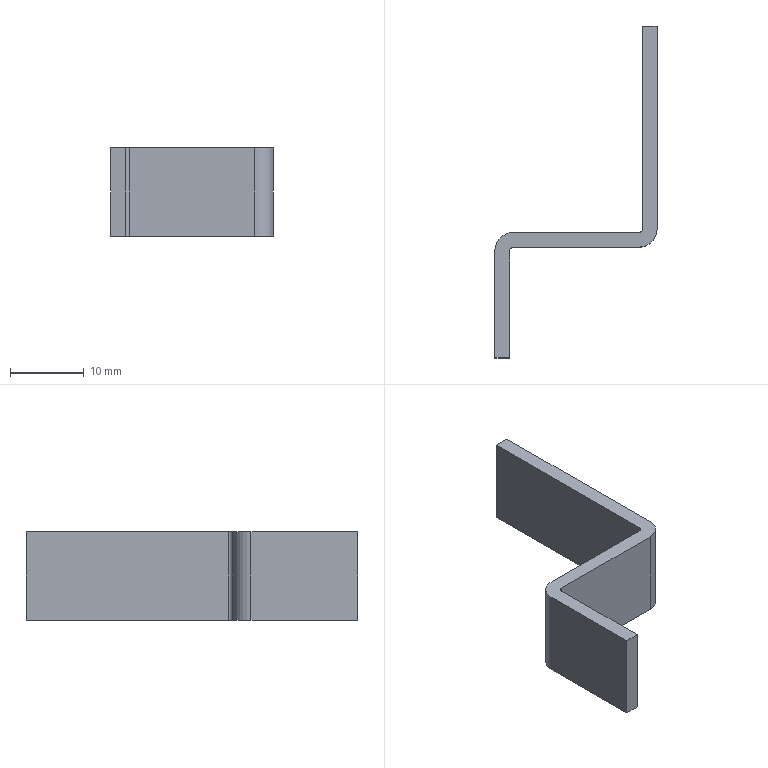Part | STEP file | Clip | 1 solid | 14 faces | box 22 x 45 x 12 mm | volume 1529 mm3 | plane 10 | cylinder 4 | commonest cylinder face diameters 1 x2 5 x2
STEP:
#1=CARTESIAN_POINT('',(0.,-1.053,12.));
#2=VERTEX_POINT('',#1);
#3=CARTESIAN_POINT('',(0.,-28.553,12.));
#4=VERTEX_POINT('',#3);
#5=CARTESIAN_POINT('',(0.,-1.053,12.));
#6=DIRECTION('',(0.,-1.,0.));
#7=VECTOR('',#6,1000.);
#8=LINE('',#5,#7);
#9=EDGE_CURVE('',#2,#4,#8,.T.);
#10=ORIENTED_EDGE('',*,*,#9,.T.);
#11=CARTESIAN_POINT('',(0.,-28.553,0.));
#12=VERTEX_POINT('',#11);
#13=CARTESIAN_POINT('',(0.,-28.553,12.));
#14=DIRECTION('',(0.,0.,-1.));
#15=VECTOR('',#14,1000.);
#16=LINE('',#13,#15);
#17=EDGE_CURVE('',#4,#12,#16,.T.);
#18=ORIENTED_EDGE('',*,*,#17,.T.);
#19=CARTESIAN_POINT('',(0.,-1.053,0.));
#20=VERTEX_POINT('',#19);
#21=CARTESIAN_POINT('',(0.,-1.053,0.));
#22=DIRECTION('',(0.,1.,0.));
#23=VECTOR('',#22,1000.);
#24=LINE('',#21,#23);
#25=EDGE_CURVE('',#12,#20,#24,.T.);
#26=ORIENTED_EDGE('',*,*,#25,.T.);
#27=CARTESIAN_POINT('',(0.,-1.053,12.));
#28=DIRECTION('',(0.,0.,1.));
#29=VECTOR('',#28,1000.);
#30=LINE('',#27,#29);
#31=EDGE_CURVE('',#20,#2,#30,.T.);
#32=ORIENTED_EDGE('',*,*,#31,.T.);
#33=EDGE_LOOP('',(#10,#18,#26,#32));
#34=FACE_OUTER_BOUND('',#33,.T.);
#35=CARTESIAN_POINT('',(0.,-1.053,12.));
#36=DIRECTION('',(1.,0.,0.));
#37=DIRECTION('',(0.,1.,0.));
#38=AXIS2_PLACEMENT_3D('',#35,#36,#37);
#39=PLANE('',#38);
#40=ADVANCED_FACE('',(#34),#39,.T.);
#41=CARTESIAN_POINT('',(-2.5,-31.053,12.));
#42=VERTEX_POINT('',#41);
#43=CARTESIAN_POINT('',(-2.5,-28.553,12.));
#44=DIRECTION('',(0.,0.,-1.));
#45=DIRECTION('',(-1.,0.,0.));
#46=AXIS2_PLACEMENT_3D('',#43,#44,#45);
#47=CIRCLE('',#46,2.5);
#48=EDGE_CURVE('',#4,#42,#47,.T.);
#49=ORIENTED_EDGE('',*,*,#48,.T.);
#50=CARTESIAN_POINT('',(-2.5,-31.053,0.));
#51=VERTEX_POINT('',#50);
#52=CARTESIAN_POINT('',(-2.5,-31.053,12.));
#53=DIRECTION('',(0.,0.,-1.));
#54=VECTOR('',#53,1000.);
#55=LINE('',#52,#54);
#56=EDGE_CURVE('',#42,#51,#55,.T.);
#57=ORIENTED_EDGE('',*,*,#56,.T.);
#58=CARTESIAN_POINT('',(-2.5,-28.553,0.));
#59=DIRECTION('',(0.,0.,1.));
#60=DIRECTION('',(-1.,0.,0.));
#61=AXIS2_PLACEMENT_3D('',#58,#59,#60);
#62=CIRCLE('',#61,2.5);
#63=EDGE_CURVE('',#51,#12,#62,.T.);
#64=ORIENTED_EDGE('',*,*,#63,.T.);
#65=ORIENTED_EDGE('',*,*,#17,.F.);
#66=EDGE_LOOP('',(#49,#57,#64,#65));
#67=FACE_OUTER_BOUND('',#66,.T.);
#68=CARTESIAN_POINT('',(-2.5,-28.553,12.));
#69=DIRECTION('',(0.,0.,-1.));
#70=DIRECTION('',(-1.,0.,0.));
#71=AXIS2_PLACEMENT_3D('',#68,#69,#70);
#72=CYLINDRICAL_SURFACE('',#71,2.5);
#73=ADVANCED_FACE('',(#67),#72,.T.);
#74=CARTESIAN_POINT('',(-2.,-28.553,12.));
#75=VERTEX_POINT('',#74);
#76=CARTESIAN_POINT('',(-2.,-1.053,12.));
#77=VERTEX_POINT('',#76);
#78=CARTESIAN_POINT('',(-2.,-31.553,12.));
#79=DIRECTION('',(0.,1.,0.));
#80=VECTOR('',#79,1000.);
#81=LINE('',#78,#80);
#82=EDGE_CURVE('',#75,#77,#81,.T.);
#83=ORIENTED_EDGE('',*,*,#82,.F.);
#84=CARTESIAN_POINT('',(-2.5,-29.053,12.));
#85=VERTEX_POINT('',#84);
#86=CARTESIAN_POINT('',(-2.5,-28.553,12.));
#87=DIRECTION('',(0.,0.,-1.));
#88=DIRECTION('',(-1.,0.,0.));
#89=AXIS2_PLACEMENT_3D('',#86,#87,#88);
#90=CIRCLE('',#89,0.5);
#91=EDGE_CURVE('',#75,#85,#90,.T.);
#92=ORIENTED_EDGE('',*,*,#91,.T.);
#93=CARTESIAN_POINT('',(-19.5,-29.053,12.));
#94=VERTEX_POINT('',#93);
#95=CARTESIAN_POINT('',(-2.,-29.053,12.));
#96=DIRECTION('',(-1.,0.,0.));
#97=VECTOR('',#96,1000.);
#98=LINE('',#95,#97);
#99=EDGE_CURVE('',#85,#94,#98,.T.);
#100=ORIENTED_EDGE('',*,*,#99,.T.);
#101=CARTESIAN_POINT('',(-22.,-31.553,12.));
#102=VERTEX_POINT('',#101);
#103=CARTESIAN_POINT('',(-19.5,-31.553,12.));
#104=DIRECTION('',(0.,0.,1.));
#105=DIRECTION('',(-1.,0.,0.));
#106=AXIS2_PLACEMENT_3D('',#103,#104,#105);
#107=CIRCLE('',#106,2.5);
#108=EDGE_CURVE('',#94,#102,#107,.T.);
#109=ORIENTED_EDGE('',*,*,#108,.T.);
#110=CARTESIAN_POINT('',(-22.,-46.053,12.));
#111=VERTEX_POINT('',#110);
#112=CARTESIAN_POINT('',(-22.,-29.053,12.));
#113=DIRECTION('',(0.,-1.,0.));
#114=VECTOR('',#113,1000.);
#115=LINE('',#112,#114);
#116=EDGE_CURVE('',#102,#111,#115,.T.);
#117=ORIENTED_EDGE('',*,*,#116,.T.);
#118=CARTESIAN_POINT('',(-20.,-46.053,12.));
#119=VERTEX_POINT('',#118);
#120=CARTESIAN_POINT('',(-20.,-46.053,12.));
#121=DIRECTION('',(-1.,0.,0.));
#122=VECTOR('',#121,1000.);
#123=LINE('',#120,#122);
#124=EDGE_CURVE('',#119,#111,#123,.T.);
#125=ORIENTED_EDGE('',*,*,#124,.F.);
#126=CARTESIAN_POINT('',(-20.,-31.553,12.));
#127=VERTEX_POINT('',#126);
#128=CARTESIAN_POINT('',(-20.,-31.053,12.));
#129=DIRECTION('',(0.,-1.,0.));
#130=VECTOR('',#129,1000.);
#131=LINE('',#128,#130);
#132=EDGE_CURVE('',#127,#119,#131,.T.);
#133=ORIENTED_EDGE('',*,*,#132,.F.);
#134=CARTESIAN_POINT('',(-19.5,-31.053,12.));
#135=VERTEX_POINT('',#134);
#136=CARTESIAN_POINT('',(-19.5,-31.553,12.));
#137=DIRECTION('',(0.,0.,-1.));
#138=DIRECTION('',(-1.,0.,0.));
#139=AXIS2_PLACEMENT_3D('',#136,#137,#138);
#140=CIRCLE('',#139,0.5);
#141=EDGE_CURVE('',#127,#135,#140,.T.);
#142=ORIENTED_EDGE('',*,*,#141,.T.);
#143=CARTESIAN_POINT('',(-20.,-31.053,12.));
#144=DIRECTION('',(-1.,0.,0.));
#145=VECTOR('',#144,1000.);
#146=LINE('',#143,#145);
#147=EDGE_CURVE('',#42,#135,#146,.T.);
#148=ORIENTED_EDGE('',*,*,#147,.F.);
#149=ORIENTED_EDGE('',*,*,#48,.F.);
#150=ORIENTED_EDGE('',*,*,#9,.F.);
#151=CARTESIAN_POINT('',(-19.5,-1.053,12.));
#152=DIRECTION('',(1.,0.,0.));
#153=VECTOR('',#152,1000.);
#154=LINE('',#151,#153);
#155=EDGE_CURVE('',#77,#2,#154,.T.);
#156=ORIENTED_EDGE('',*,*,#155,.F.);
#157=EDGE_LOOP('',(#83,#92,#100,#109,#117,#125,#133,#142,#148,#149,#150,#156));
#158=FACE_OUTER_BOUND('',#157,.T.);
#159=CARTESIAN_POINT('',(-19.5,-31.553,12.));
#160=DIRECTION('',(0.,0.,-1.));
#161=DIRECTION('',(-1.,0.,0.));
#162=AXIS2_PLACEMENT_3D('',#159,#160,#161);
#163=PLANE('',#162);
#164=ADVANCED_FACE('',(#158),#163,.F.);
#165=ORIENTED_EDGE('',*,*,#155,.T.);
#166=ORIENTED_EDGE('',*,*,#31,.F.);
#167=CARTESIAN_POINT('',(-2.,-1.053,0.));
#168=VERTEX_POINT('',#167);
#169=CARTESIAN_POINT('',(-2.,-1.053,0.));
#170=DIRECTION('',(-1.,0.,0.));
#171=VECTOR('',#170,1000.);
#172=LINE('',#169,#171);
#173=EDGE_CURVE('',#20,#168,#172,.T.);
#174=ORIENTED_EDGE('',*,*,#173,.T.);
#175=CARTESIAN_POINT('',(-2.,-1.053,12.));
#176=DIRECTION('',(0.,0.,1.));
#177=VECTOR('',#176,1000.);
#178=LINE('',#175,#177);
#179=EDGE_CURVE('',#168,#77,#178,.T.);
#180=ORIENTED_EDGE('',*,*,#179,.T.);
#181=EDGE_LOOP('',(#165,#166,#174,#180));
#182=FACE_OUTER_BOUND('',#181,.T.);
#183=CARTESIAN_POINT('',(-2.,-1.053,12.));
#184=DIRECTION('',(0.,1.,0.));
#185=DIRECTION('',(-1.,0.,0.));
#186=AXIS2_PLACEMENT_3D('',#183,#184,#185);
#187=PLANE('',#186);
#188=ADVANCED_FACE('',(#182),#187,.T.);
#189=CARTESIAN_POINT('',(-2.,-28.553,0.));
#190=VERTEX_POINT('',#189);
#191=CARTESIAN_POINT('',(-2.,-29.053,0.));
#192=DIRECTION('',(0.,1.,0.));
#193=VECTOR('',#192,1000.);
#194=LINE('',#191,#193);
#195=EDGE_CURVE('',#190,#168,#194,.T.);
#196=ORIENTED_EDGE('',*,*,#195,.T.);
#197=ORIENTED_EDGE('',*,*,#173,.F.);
#198=ORIENTED_EDGE('',*,*,#25,.F.);
#199=ORIENTED_EDGE('',*,*,#63,.F.);
#200=CARTESIAN_POINT('',(-19.5,-31.053,0.));
#201=VERTEX_POINT('',#200);
#202=CARTESIAN_POINT('',(-20.,-31.053,0.));
#203=DIRECTION('',(1.,0.,0.));
#204=VECTOR('',#203,1000.);
#205=LINE('',#202,#204);
#206=EDGE_CURVE('',#201,#51,#205,.T.);
#207=ORIENTED_EDGE('',*,*,#206,.F.);
#208=CARTESIAN_POINT('',(-20.,-31.553,0.));
#209=VERTEX_POINT('',#208);
#210=CARTESIAN_POINT('',(-19.5,-31.553,0.));
#211=DIRECTION('',(0.,0.,1.));
#212=DIRECTION('',(-1.,0.,0.));
#213=AXIS2_PLACEMENT_3D('',#210,#211,#212);
#214=CIRCLE('',#213,0.5);
#215=EDGE_CURVE('',#201,#209,#214,.T.);
#216=ORIENTED_EDGE('',*,*,#215,.T.);
#217=CARTESIAN_POINT('',(-20.,-46.053,0.));
#218=VERTEX_POINT('',#217);
#219=CARTESIAN_POINT('',(-20.,-31.053,0.));
#220=DIRECTION('',(0.,1.,0.));
#221=VECTOR('',#220,1000.);
#222=LINE('',#219,#221);
#223=EDGE_CURVE('',#218,#209,#222,.T.);
#224=ORIENTED_EDGE('',*,*,#223,.F.);
#225=CARTESIAN_POINT('',(-22.,-46.053,0.));
#226=VERTEX_POINT('',#225);
#227=CARTESIAN_POINT('',(-20.,-46.053,0.));
#228=DIRECTION('',(1.,0.,0.));
#229=VECTOR('',#228,1000.);
#230=LINE('',#227,#229);
#231=EDGE_CURVE('',#226,#218,#230,.T.);
#232=ORIENTED_EDGE('',*,*,#231,.F.);
#233=CARTESIAN_POINT('',(-22.,-31.553,0.));
#234=VERTEX_POINT('',#233);
#235=CARTESIAN_POINT('',(-22.,-31.553,0.));
#236=DIRECTION('',(0.,1.,0.));
#237=VECTOR('',#236,1000.);
#238=LINE('',#235,#237);
#239=EDGE_CURVE('',#226,#234,#238,.T.);
#240=ORIENTED_EDGE('',*,*,#239,.T.);
#241=CARTESIAN_POINT('',(-19.5,-29.053,0.));
#242=VERTEX_POINT('',#241);
#243=CARTESIAN_POINT('',(-19.5,-31.553,0.));
#244=DIRECTION('',(0.,0.,-1.));
#245=DIRECTION('',(-1.,0.,0.));
#246=AXIS2_PLACEMENT_3D('',#243,#244,#245);
#247=CIRCLE('',#246,2.5);
#248=EDGE_CURVE('',#234,#242,#247,.T.);
#249=ORIENTED_EDGE('',*,*,#248,.T.);
#250=CARTESIAN_POINT('',(-2.5,-29.053,0.));
#251=VERTEX_POINT('',#250);
#252=CARTESIAN_POINT('',(-22.,-29.053,0.));
#253=DIRECTION('',(1.,0.,0.));
#254=VECTOR('',#253,1000.);
#255=LINE('',#252,#254);
#256=EDGE_CURVE('',#242,#251,#255,.T.);
#257=ORIENTED_EDGE('',*,*,#256,.T.);
#258=CARTESIAN_POINT('',(-2.5,-28.553,0.));
#259=DIRECTION('',(0.,0.,1.));
#260=DIRECTION('',(-1.,0.,0.));
#261=AXIS2_PLACEMENT_3D('',#258,#259,#260);
#262=CIRCLE('',#261,0.5);
#263=EDGE_CURVE('',#251,#190,#262,.T.);
#264=ORIENTED_EDGE('',*,*,#263,.T.);
#265=EDGE_LOOP('',(#196,#197,#198,#199,#207,#216,#224,#232,#240,#249,#257,#264));
#266=FACE_OUTER_BOUND('',#265,.T.);
#267=CARTESIAN_POINT('',(-2.5,-29.053,0.));
#268=DIRECTION('',(0.,0.,-1.));
#269=DIRECTION('',(-1.,0.,0.));
#270=AXIS2_PLACEMENT_3D('',#267,#268,#269);
#271=PLANE('',#270);
#272=ADVANCED_FACE('',(#266),#271,.T.);
#273=ORIENTED_EDGE('',*,*,#147,.T.);
#274=CARTESIAN_POINT('',(-19.5,-31.053,12.));
#275=DIRECTION('',(0.,0.,-1.));
#276=VECTOR('',#275,1000.);
#277=LINE('',#274,#276);
#278=EDGE_CURVE('',#135,#201,#277,.T.);
#279=ORIENTED_EDGE('',*,*,#278,.T.);
#280=ORIENTED_EDGE('',*,*,#206,.T.);
#281=ORIENTED_EDGE('',*,*,#56,.F.);
#282=EDGE_LOOP('',(#273,#279,#280,#281));
#283=FACE_OUTER_BOUND('',#282,.T.);
#284=CARTESIAN_POINT('',(-20.,-31.053,12.));
#285=DIRECTION('',(0.,-1.,0.));
#286=DIRECTION('',(0.,0.,-1.));
#287=AXIS2_PLACEMENT_3D('',#284,#285,#286);
#288=PLANE('',#287);
#289=ADVANCED_FACE('',(#283),#288,.T.);
#290=CARTESIAN_POINT('',(-2.,-28.553,12.));
#291=DIRECTION('',(0.,0.,-1.));
#292=VECTOR('',#291,1000.);
#293=LINE('',#290,#292);
#294=EDGE_CURVE('',#75,#190,#293,.T.);
#295=ORIENTED_EDGE('',*,*,#294,.F.);
#296=ORIENTED_EDGE('',*,*,#82,.T.);
#297=ORIENTED_EDGE('',*,*,#179,.F.);
#298=ORIENTED_EDGE('',*,*,#195,.F.);
#299=EDGE_LOOP('',(#295,#296,#297,#298));
#300=FACE_OUTER_BOUND('',#299,.T.);
#301=CARTESIAN_POINT('',(-2.,-1.053,12.));
#302=DIRECTION('',(1.,0.,0.));
#303=DIRECTION('',(0.,1.,0.));
#304=AXIS2_PLACEMENT_3D('',#301,#302,#303);
#305=PLANE('',#304);
#306=ADVANCED_FACE('',(#300),#305,.F.);
#307=ORIENTED_EDGE('',*,*,#278,.F.);
#308=ORIENTED_EDGE('',*,*,#141,.F.);
#309=CARTESIAN_POINT('',(-20.,-31.553,12.));
#310=DIRECTION('',(0.,0.,1.));
#311=VECTOR('',#310,1000.);
#312=LINE('',#309,#311);
#313=EDGE_CURVE('',#209,#127,#312,.T.);
#314=ORIENTED_EDGE('',*,*,#313,.F.);
#315=ORIENTED_EDGE('',*,*,#215,.F.);
#316=EDGE_LOOP('',(#307,#308,#314,#315));
#317=FACE_OUTER_BOUND('',#316,.T.);
#318=CARTESIAN_POINT('',(-19.5,-31.553,12.));
#319=DIRECTION('',(0.,0.,-1.));
#320=DIRECTION('',(-1.,0.,0.));
#321=AXIS2_PLACEMENT_3D('',#318,#319,#320);
#322=CYLINDRICAL_SURFACE('',#321,0.5);
#323=ADVANCED_FACE('',(#317),#322,.F.);
#324=CARTESIAN_POINT('',(-2.5,-29.053,12.));
#325=DIRECTION('',(0.,0.,-1.));
#326=VECTOR('',#325,1000.);
#327=LINE('',#324,#326);
#328=EDGE_CURVE('',#85,#251,#327,.T.);
#329=ORIENTED_EDGE('',*,*,#328,.F.);
#330=ORIENTED_EDGE('',*,*,#91,.F.);
#331=ORIENTED_EDGE('',*,*,#294,.T.);
#332=ORIENTED_EDGE('',*,*,#263,.F.);
#333=EDGE_LOOP('',(#329,#330,#331,#332));
#334=FACE_OUTER_BOUND('',#333,.T.);
#335=CARTESIAN_POINT('',(-2.5,-28.553,12.));
#336=DIRECTION('',(0.,0.,-1.));
#337=DIRECTION('',(-1.,0.,0.));
#338=AXIS2_PLACEMENT_3D('',#335,#336,#337);
#339=CYLINDRICAL_SURFACE('',#338,0.5);
#340=ADVANCED_FACE('',(#334),#339,.F.);
#341=ORIENTED_EDGE('',*,*,#132,.T.);
#342=CARTESIAN_POINT('',(-20.,-46.053,12.));
#343=DIRECTION('',(0.,0.,-1.));
#344=VECTOR('',#343,1000.);
#345=LINE('',#342,#344);
#346=EDGE_CURVE('',#119,#218,#345,.T.);
#347=ORIENTED_EDGE('',*,*,#346,.T.);
#348=ORIENTED_EDGE('',*,*,#223,.T.);
#349=ORIENTED_EDGE('',*,*,#313,.T.);
#350=EDGE_LOOP('',(#341,#347,#348,#349));
#351=FACE_OUTER_BOUND('',#350,.T.);
#352=CARTESIAN_POINT('',(-20.,-31.053,12.));
#353=DIRECTION('',(1.,0.,0.));
#354=DIRECTION('',(0.,1.,0.));
#355=AXIS2_PLACEMENT_3D('',#352,#353,#354);
#356=PLANE('',#355);
#357=ADVANCED_FACE('',(#351),#356,.T.);
#358=CARTESIAN_POINT('',(-19.5,-29.053,12.));
#359=DIRECTION('',(0.,0.,-1.));
#360=VECTOR('',#359,1000.);
#361=LINE('',#358,#360);
#362=EDGE_CURVE('',#94,#242,#361,.T.);
#363=ORIENTED_EDGE('',*,*,#362,.F.);
#364=ORIENTED_EDGE('',*,*,#99,.F.);
#365=ORIENTED_EDGE('',*,*,#328,.T.);
#366=ORIENTED_EDGE('',*,*,#256,.F.);
#367=EDGE_LOOP('',(#363,#364,#365,#366));
#368=FACE_OUTER_BOUND('',#367,.T.);
#369=CARTESIAN_POINT('',(-20.,-29.053,12.));
#370=DIRECTION('',(0.,-1.,0.));
#371=DIRECTION('',(0.,0.,-1.));
#372=AXIS2_PLACEMENT_3D('',#369,#370,#371);
#373=PLANE('',#372);
#374=ADVANCED_FACE('',(#368),#373,.F.);
#375=ORIENTED_EDGE('',*,*,#124,.T.);
#376=CARTESIAN_POINT('',(-22.,-46.053,12.));
#377=DIRECTION('',(0.,0.,-1.));
#378=VECTOR('',#377,1000.);
#379=LINE('',#376,#378);
#380=EDGE_CURVE('',#111,#226,#379,.T.);
#381=ORIENTED_EDGE('',*,*,#380,.T.);
#382=ORIENTED_EDGE('',*,*,#231,.T.);
#383=ORIENTED_EDGE('',*,*,#346,.F.);
#384=EDGE_LOOP('',(#375,#381,#382,#383));
#385=FACE_OUTER_BOUND('',#384,.T.);
#386=CARTESIAN_POINT('',(-20.,-46.053,12.));
#387=DIRECTION('',(0.,-1.,0.));
#388=DIRECTION('',(0.,0.,-1.));
#389=AXIS2_PLACEMENT_3D('',#386,#387,#388);
#390=PLANE('',#389);
#391=ADVANCED_FACE('',(#385),#390,.T.);
#392=ORIENTED_EDGE('',*,*,#108,.F.);
#393=ORIENTED_EDGE('',*,*,#362,.T.);
#394=ORIENTED_EDGE('',*,*,#248,.F.);
#395=CARTESIAN_POINT('',(-22.,-31.553,12.));
#396=DIRECTION('',(0.,0.,1.));
#397=VECTOR('',#396,1000.);
#398=LINE('',#395,#397);
#399=EDGE_CURVE('',#234,#102,#398,.T.);
#400=ORIENTED_EDGE('',*,*,#399,.T.);
#401=EDGE_LOOP('',(#392,#393,#394,#400));
#402=FACE_OUTER_BOUND('',#401,.T.);
#403=CARTESIAN_POINT('',(-19.5,-31.553,12.));
#404=DIRECTION('',(0.,0.,-1.));
#405=DIRECTION('',(-1.,0.,0.));
#406=AXIS2_PLACEMENT_3D('',#403,#404,#405);
#407=CYLINDRICAL_SURFACE('',#406,2.5);
#408=ADVANCED_FACE('',(#402),#407,.T.);
#409=ORIENTED_EDGE('',*,*,#380,.F.);
#410=ORIENTED_EDGE('',*,*,#116,.F.);
#411=ORIENTED_EDGE('',*,*,#399,.F.);
#412=ORIENTED_EDGE('',*,*,#239,.F.);
#413=EDGE_LOOP('',(#409,#410,#411,#412));
#414=FACE_OUTER_BOUND('',#413,.T.);
#415=CARTESIAN_POINT('',(-22.,-31.053,12.));
#416=DIRECTION('',(1.,0.,0.));
#417=DIRECTION('',(0.,1.,0.));
#418=AXIS2_PLACEMENT_3D('',#415,#416,#417);
#419=PLANE('',#418);
#420=ADVANCED_FACE('',(#414),#419,.F.);
#421=CLOSED_SHELL('',(#40,#73,#164,#188,#272,#289,#306,#323,#340,#357,#374,#391,#408,#420));
#422=MANIFOLD_SOLID_BREP('',#421);
#423=CARTESIAN_POINT('',(0.,0.,0.));
#424=DIRECTION('',(0.,0.,1.));
#425=DIRECTION('',(1.,0.,0.));
#426=AXIS2_PLACEMENT_3D('',#423,#424,#425);
#427=(LENGTH_UNIT()NAMED_UNIT(*)SI_UNIT(.MILLI.,.METRE.));
#428=UNCERTAINTY_MEASURE_WITH_UNIT(LENGTH_MEASURE(0.00001),#427,'','');
#429=(NAMED_UNIT(*)PLANE_ANGLE_UNIT()SI_UNIT($,.RADIAN.));
#430=(NAMED_UNIT(*)SI_UNIT($,.STERADIAN.)SOLID_ANGLE_UNIT());
#431=(GEOMETRIC_REPRESENTATION_CONTEXT(3)GLOBAL_UNCERTAINTY_ASSIGNED_CONTEXT((#428))GLOBAL_UNIT_ASSIGNED_CONTEXT((#427,#429,#430))REPRESENTATION_CONTEXT('',''));
#432=ADVANCED_BREP_SHAPE_REPRESENTATION('',(#422,#426),#431);